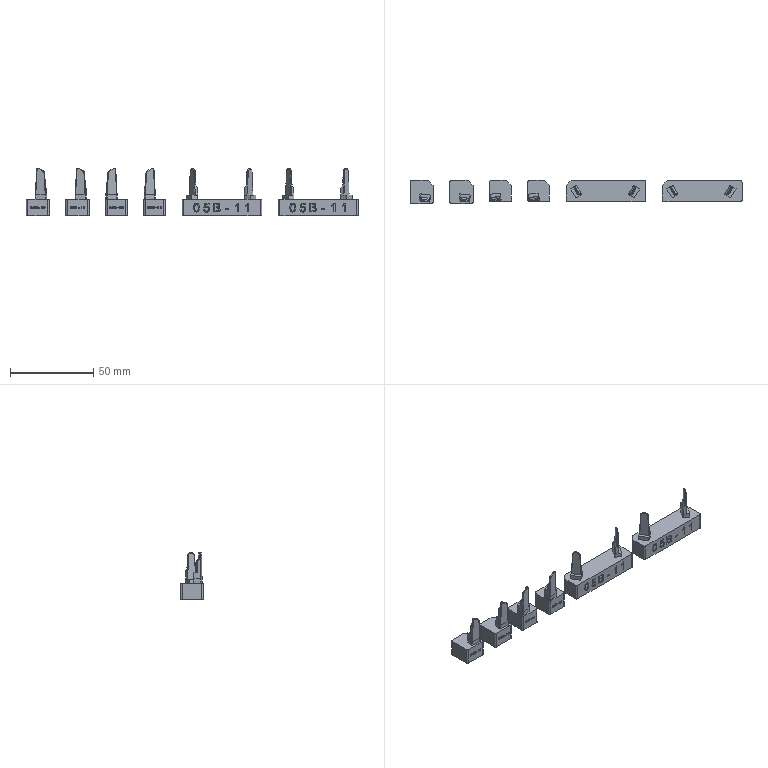NC program | NX | posted with a generic post | part box 200 x 14 x 28.763 mm
Lines 21030 to 21844 of 209396:
(CONTOUR_AREA_0_0 , TOOL : D4R2)
N41980 M6
N41982 G53
N41984 G17 G0 G90 X91.621 Y3.419 S13000 M3
N41986 G43 Z5. H0
N41988 Z2.6
N41990 G94 G1 Z-4.451 F2000.
N41992 X91.634 Y3.432 Z-4.51
N41994 X91.669 Y3.467 Z-4.546
N41996 X91.713 Y3.511 Z-4.547
N41998 X91.748 Y3.546 Z-4.511
N42000 X91.762 Y3.56 Z-4.453
N42002 X91.765 Y3.563 Z-4.28
N42004 X91.773 Y3.571 Z-4.083
N42006 X91.781 Y3.579 Z-3.96
N42008 X91.784 Y3.582 Z-3.927
N42010 X91.805 Y3.603 Z-3.742
N42012 X91.841 Y3.639 Z-3.608
N42014 X91.875 Y3.673 Z-3.541
N42016 X91.909 Y3.707 Z-3.499
N42018 X91.942 Y3.74 Z-3.477
N42020 X91.976 Y3.774 Z-3.468
N42022 X92.043 Y3.841 Z-3.476
N42024 X92.111 Y3.909 Z-3.512
N42026 X92.178 Y3.976 Z-3.582
N42028 X92.246 Y4.044 Z-3.679
N42030 X92.313 Y4.111 Z-3.817
N42032 X92.347 Y4.145 Z-3.917
N42034 X92.38 Y4.178 Z-4.052
N42036 X92.404 Y4.202 Z-4.2
N42038 X92.412 Y4.21 Z-4.274
N42040 X92.422 Y4.22 Z-4.414
N42042 X92.45 Y4.239 Z-4.413
N42044 X92.594 Y4.321 Z-4.406
N42046 X92.579 Y4.307 Z-4.211
N42048 X92.564 Y4.292 Z-4.076
N42050 X92.521 Y4.249 Z-3.857
N42052 X92.478 Y4.206 Z-3.71
N42054 X92.392 Y4.12 Z-3.503
N42056 X92.306 Y4.034 Z-3.355
N42058 X92.22 Y3.948 Z-3.244
N42060 X92.134 Y3.862 Z-3.165
N42062 X92.048 Y3.776 Z-3.112
N42064 X91.962 Y3.69 Z-3.083
N42066 X91.876 Y3.604 Z-3.088
N42068 X91.826 Y3.554 Z-3.107
N42070 X91.776 Y3.504 Z-3.15
N42072 X91.726 Y3.454 Z-3.23
N42074 X91.701 Y3.429 Z-3.298
N42076 X91.676 Y3.404 Z-3.435
N42078 X91.67 Y3.398 Z-3.487
N42080 X91.666 Y3.393 Z-3.539
N42082 X91.664 Y3.391 Z-3.578
N42084 X91.643 Y3.371 Z-4.292
N42086 X91.608 Y3.31 Z-3.934
N42088 X91.572 Y3.25 Z-3.74
N42090 X91.542 Y3.199 Z-3.628
N42092 X91.55 Y3.208 Z-3.334
N42094 X91.554 Y3.212 Z-3.226
N42096 X91.558 Y3.216 Z-3.182
N42098 X91.575 Y3.232 Z-3.081
N42100 X91.596 Y3.253 Z-3.008
N42102 X91.617 Y3.274 Z-2.962
N42104 X91.659 Y3.316 Z-2.898
N42106 X91.701 Y3.359 Z-2.856
N42108 X91.743 Y3.401 Z-2.83
N42110 X91.827 Y3.485 Z-2.805
N42112 X91.911 Y3.569
N42114 X92.011 Y3.668 Z-2.832
N42116 X92.11 Y3.767 Z-2.882
N42118 X92.209 Y3.866 Z-2.959
N42120 X92.308 Y3.965 Z-3.062
N42122 X92.407 Y4.065 Z-3.196
N42124 X92.506 Y4.164 Z-3.373
N42126 X92.605 Y4.263 Z-3.622
N42128 X92.655 Y4.312 Z-3.8
N42130 X92.679 Y4.337 Z-3.915
N42132 X92.704 Y4.362 Z-4.078
N42134 X92.727 Y4.385 Z-4.401
N42136 X92.775 Y4.407 Z-4.398
N42138 X92.847 Y4.435 Z-4.394
N42140 X92.828 Y4.416 Z-4.117
N42142 X92.795 Y4.383 Z-3.873
N42144 X92.742 Y4.33 Z-3.642
N42146 X92.689 Y4.277 Z-3.472
N42148 X92.636 Y4.223 Z-3.338
N42150 X92.583 Y4.17 Z-3.225
N42152 X92.477 Y4.064 Z-3.043
N42154 X92.371 Y3.958 Z-2.9
N42156 X92.265 Y3.852 Z-2.788
N42158 X92.159 Y3.746 Z-2.703
N42160 X92.053 Y3.64 Z-2.64
N42162 X91.947 Y3.534 Z-2.599
N42164 X91.826 Y3.413 Z-2.581
N42166 X91.705 Y3.293 Z-2.597
N42168 X91.645 Y3.232 Z-2.623
N42170 X91.584 Y3.172 Z-2.663
N42172 X91.524 Y3.112 Z-2.734
N42174 X91.494 Y3.081 Z-2.785
N42176 X91.464 Y3.051 Z-2.866
N42178 X91.455 Y3.043 Z-2.904
N42180 X91.447 Y3.034 Z-2.952
N42182 X91.438 Y3.026 Z-3.034
N42184 X91.43 Y3.017 Z-3.328
N42186 X91.315 Y2.833 Z-3.126
N42188 X91.322 Y2.839 Z-2.897
N42190 X91.324 Y2.841 Z-2.857
N42192 X91.332 Y2.85 Z-2.792
N42194 X91.349 Y2.867 Z-2.714
N42196 X91.389 Y2.906 Z-2.62
N42198 X91.428 Y2.946 Z-2.559
N42200 X91.507 Y3.025 Z-2.481
N42202 X91.586 Y3.104 Z-2.435
N42204 X91.665 Y3.183 Z-2.408
N42206 X91.744 Y3.262 Z-2.398
N42208 X91.824 Y3.341 Z-2.399
N42210 X91.982 Y3.499 Z-2.434
N42212 X92.088 Y3.605 Z-2.48
N42214 X92.194 Y3.711 Z-2.545
N42216 X92.3 Y3.817 Z-2.631
N42218 X92.406 Y3.923 Z-2.737
N42220 X92.512 Y4.029 Z-2.87
N42222 X92.618 Y4.135 Z-3.034
N42224 X92.724 Y4.241 Z-3.249
N42226 X92.777 Y4.294 Z-3.381
N42228 X92.83 Y4.347 Z-3.54
N42230 X92.883 Y4.4 Z-3.746
N42232 X92.909 Y4.426 Z-3.885
N42234 X92.935 Y4.453 Z-4.092
N42236 X92.951 Y4.468 Z-4.389
N42238 X93.048 Y4.495 Z-4.386
N42240 X93.032 Y4.479 Z-4.054
N42242 X92.99 Y4.438 Z-3.77
N42244 X92.949 Y4.396 Z-3.582
N42246 X92.865 Y4.312 Z-3.315
N42248 X92.759 Y4.206 Z-3.067
N42250 X92.653 Y4.1 Z-2.875
N42252 X92.547 Y3.994 Z-2.722
N42254 X92.441 Y3.888 Z-2.597
N42256 X92.335 Y3.782 Z-2.494
N42258 X92.229 Y3.676 Z-2.411
N42260 X92.123 Y3.57 Z-2.344
N42262 X92.017 Y3.464 Z-2.294
N42264 X91.919 Y3.366 Z-2.263
N42266 X91.821 Y3.268 Z-2.244
N42268 X91.723 Y3.17 Z-2.239
N42270 X91.625 Y3.072 Z-2.251
N42272 X91.527 Y2.974 Z-2.279
N42274 X91.429 Y2.876 Z-2.333
N42276 X91.331 Y2.778 Z-2.422
N42278 X91.282 Y2.729 Z-2.493
N42280 X91.233 Y2.68 Z-2.603
N42282 X91.214 Y2.661 Z-2.691
N42284 X91.207 Y2.654 Z-2.739
N42286 X91.198 Y2.646 Z-2.999
N42288 X91.126 Y2.531 Z-2.946
N42290 X91.081 Y2.458 Z-2.916
N42292 X91.087 Y2.464 Z-2.689
N42294 X91.089 Y2.466 Z-2.66
N42296 X91.098 Y2.475 Z-2.603
N42298 X91.115 Y2.492 Z-2.527
N42300 X91.159 Y2.536 Z-2.423
N42302 X91.203 Y2.58 Z-2.352
N42304 X91.256 Y2.633 Z-2.289
N42306 X91.309 Y2.686 Z-2.242
N42308 X91.415 Y2.792 Z-2.172
N42310 X91.521 Y2.898 Z-2.13
N42312 X91.628 Y3.005 Z-2.107
N42314 X91.734 Y3.111 Z-2.102
N42316 X91.84 Y3.217 Z-2.111
N42318 X91.946 Y3.323 Z-2.134
N42320 X92.052 Y3.429 Z-2.172
N42322 X92.158 Y3.535 Z-2.224
N42324 X92.264 Y3.641 Z-2.29
N42326 X92.37 Y3.747 Z-2.372
N42328 X92.476 Y3.853 Z-2.473
N42330 X92.582 Y3.959 Z-2.592
N42332 X92.688 Y4.065 Z-2.737
N42334 X92.794 Y4.171 Z-2.914
N42336 X92.9 Y4.277 Z-3.137
N42338 X92.957 Y4.334 Z-3.283
N42340 X93.015 Y4.392 Z-3.461
N42342 X93.072 Y4.449 Z-3.689
N42344 X93.1 Y4.477 Z-3.844
N42346 X93.129 Y4.506 Z-4.08
N42348 X93.144 Y4.521 Z-4.383
N42350 X93.191 Y4.534 Z-4.382
N42352 X93.233 Y4.54 Z-4.381
N42354 X93.22 Y4.527 Z-4.118
N42356 X93.184 Y4.491 Z-3.811
N42358 X93.149 Y4.456 Z-3.624
N42360 X93.078 Y4.385 Z-3.353
N42362 X93.007 Y4.313 Z-3.151
N42364 X92.935 Y4.242 Z-2.985
N42366 X92.829 Y4.136 Z-2.782
N42368 X92.723 Y4.03 Z-2.616
N42370 X92.617 Y3.924 Z-2.477
N42372 X92.511 Y3.818 Z-2.361
N42374 X92.405 Y3.712 Z-2.264
N42376 X92.299 Y3.606 Z-2.182
N42378 X92.193 Y3.5 Z-2.115
N42380 X92.087 Y3.394 Z-2.063
N42382 X91.981 Y3.288 Z-2.023
N42384 X91.875 Y3.182 Z-1.996
N42386 X91.769 Y3.076 Z-1.981
N42388 X91.663 Y2.969
N42390 X91.557 Y2.863 Z-1.992
N42392 X91.45 Y2.757 Z-2.021
N42394 X91.344 Y2.651 Z-2.066
N42396 X91.238 Y2.545 Z-2.134
N42398 X91.118 Y2.424 Z-2.252
N42400 X91.057 Y2.364 Z-2.343
N42402 X91.027 Y2.334 Z-2.4
N42404 X90.997 Y2.304 Z-2.48
N42406 X90.979 Y2.286 Z-2.557
N42408 X90.971 Y2.277 Z-2.614
N42410 X90.968 Y2.275 Z-2.641
N42412 X90.962 Y2.269 Z-2.865
N42414 X90.896 Y2.164 Z-2.844
N42416 X90.873 Y2.128 Z-2.843
N42418 X90.842 Y2.079 Z-2.849
N42420 X90.851 Y2.087 Z-2.597
N42422 X90.857 Y2.094 Z-2.551
N42424 X90.877 Y2.114 Z-2.461
N42426 X90.927 Y2.164 Z-2.337
N42428 X90.976 Y2.213 Z-2.25
N42430 X91.075 Y2.312 Z-2.128
N42432 X91.174 Y2.411 Z-2.04
N42434 X91.273 Y2.51 Z-1.977
N42436 X91.379 Y2.616 Z-1.927
N42438 X91.486 Y2.722 Z-1.894
N42440 X91.592 Y2.828 Z-1.875
N42442 X91.698 Y2.934 Z-1.869
N42444 X91.804 Y3.04 Z-1.876
N42446 X91.91 Y3.146 Z-1.894
N42448 X92.016 Y3.253 Z-1.923
N42450 X92.122 Y3.359 Z-1.965
N42452 X92.228 Y3.465 Z-2.019
N42454 X92.334 Y3.571 Z-2.085
N42456 X92.44 Y3.677 Z-2.165
N42458 X92.546 Y3.783 Z-2.26
N42460 X92.652 Y3.889 Z-2.373
N42462 X92.758 Y3.995 Z-2.506
N42464 X92.864 Y4.101 Z-2.664
N42466 X92.97 Y4.207 Z-2.853
N42468 X93.053 Y4.29 Z-3.032
N42470 X93.136 Y4.372 Z-3.254
N42472 X93.218 Y4.455 Z-3.545
N42474 X93.26 Y4.496 Z-3.749
N42476 X93.301 Y4.538 Z-4.072
N42478 X93.314 Y4.55 Z-4.379
N42480 X93.395 Y4.561 Z-4.377
N42482 X93.382 Y4.548 Z-4.074
N42484 X93.358 Y4.525 Z-3.854
N42486 X93.335 Y4.501 Z-3.707
N42488 X93.288 Y4.454 Z-3.483
N42490 X93.194 Y4.36 Z-3.166
N42492 X93.1 Y4.266 Z-2.93
N42494 X93.006 Y4.172 Z-2.737
N42496 X92.9 Y4.066 Z-2.557
N42498 X92.793 Y3.96 Z-2.407
N42500 X92.687 Y3.854 Z-2.278
N42502 X92.581 Y3.748 Z-2.169
N42504 X92.475 Y3.642 Z-2.074
N42506 X92.369 Y3.536 Z-1.995
N42508 X92.263 Y3.43 Z-1.929
N42510 X92.157 Y3.324 Z-1.876
N42512 X91.945 Y3.111 Z-1.801
N42514 X91.733 Y2.899 Z-1.771
N42516 X91.627 Y2.793 Z-1.772
N42518 X91.521 Y2.687 Z-1.785
N42520 X91.415 Y2.581 Z-1.811
N42522 X91.309 Y2.475 Z-1.848
N42524 X91.171 Y2.337 Z-1.922
N42526 X91.033 Y2.199 Z-2.027
N42528 X90.964 Y2.13 Z-2.099
N42530 X90.895 Y2.061 Z-2.184
N42532 X90.826 Y1.992 Z-2.298
N42534 X90.791 Y1.958 Z-2.371
N42536 X90.757 Y1.923 Z-2.47
N42538 X90.748 Y1.914 Z-2.505
N42540 X90.735 Y1.901 Z-2.577
N42542 X90.73 Y1.897 Z-2.611
N42544 X90.721 Y1.888 Z-2.86
N42546 X90.601 Y1.697 Z-2.877
N42548 X90.61 Y1.706 Z-2.634
N42550 X90.616 Y1.713 Z-2.588
N42552 X90.636 Y1.732 Z-2.494
N42554 X90.68 Y1.777 Z-2.372
N42556 X90.725 Y1.821 Z-2.28
N42558 X90.813 Y1.909 Z-2.14
N42560 X90.901 Y1.998 Z-2.031
N42562 X90.99 Y2.086 Z-1.946
N42564 X91.167 Y2.263 Z-1.82
N42566 X91.344 Y2.44 Z-1.739
N42568 X91.45 Y2.546 Z-1.707
N42570 X91.556 Y2.652 Z-1.688
N42572 X91.768 Y2.864 Z-1.681
N42574 X91.98 Y3.076 Z-1.716
N42576 X92.192 Y3.288 Z-1.792
N42578 X92.298 Y3.395 Z-1.847
N42580 X92.404 Y3.501 Z-1.913
N42582 X92.51 Y3.607 Z-1.991
N42584 X92.616 Y3.713 Z-2.083
N42586 X92.722 Y3.819 Z-2.19
N42588 X92.829 Y3.925 Z-2.315
N42590 X92.935 Y4.031 Z-2.461
N42592 X93.041 Y4.137 Z-2.633
N42594 X93.146 Y4.242 Z-2.837
N42596 X93.252 Y4.348 Z-3.093
N42598 X93.304 Y4.401 Z-3.251
N42600 X93.357 Y4.453 Z-3.44
N42602 X93.41 Y4.506 Z-3.687
N42604 X93.436 Y4.533 Z-3.856
N42606 X93.463 Y4.559 Z-4.126
N42608 X93.475 Y4.572 Z-4.374
N42610 X93.485 Y4.573
N42612 X93.547 Z-4.373
N42614 X93.536 Y4.562 Z-4.105
N42616 X93.507 Y4.533 Z-3.82
N42618 X93.478 Y4.505 Z-3.643
N42620 X93.421 Y4.447 Z-3.386
N42622 X93.363 Y4.39 Z-3.186
N42624 X93.306 Y4.332 Z-3.021
N42626 X93.191 Y4.217 Z-2.752
N42628 X93.076 Y4.102 Z-2.536
N42630 X92.97 Y3.996 Z-2.372
N42632 X92.864 Y3.89 Z-2.232
N42634 X92.758 Y3.784 Z-2.11
N42636 X92.651 Y3.678 Z-2.005
N42638 X92.545 Y3.572 Z-1.914
N42640 X92.439 Y3.466 Z-1.837
N42642 X92.227 Y3.253 Z-1.717
N42644 X92.015 Y3.041 Z-1.639
N42646 X91.803 Y2.829 Z-1.6
N42648 X91.591 Y2.617
N42650 X91.379 Y2.405 Z-1.641
N42652 X91.273 Y2.299 Z-1.679
N42654 X91.167 Y2.193 Z-1.729
N42656 X91.06 Y2.087 Z-1.792
N42658 X90.954 Y1.981 Z-1.872
N42660 X90.848 Y1.875 Z-1.971
N42662 X90.742 Y1.768 Z-2.095
N42664 X90.636 Y1.662 Z-2.248
N42666 X90.583 Y1.609 Z-2.346
N42668 X90.53 Y1.556 Z-2.472
N42670 X90.515 Y1.541 Z-2.521
N42672 X90.495 Y1.521 Z-2.615
N42674 X90.488 Y1.514 Z-2.663
N42676 X90.479 Y1.506 Z-2.916
N42678 X90.393 Y1.369 Z-2.931
N42680 X90.359 Y1.315 Z-2.939
N42682 X90.367 Y1.323 Z-2.689
N42684 X90.374 Y1.33 Z-2.642
N42686 X90.394 Y1.35 Z-2.547
N42688 X90.437 Y1.393 Z-2.428
N42690 X90.48 Y1.436 Z-2.338
N42692 X90.565 Y1.521 Z-2.198
N42694 X90.671 Y1.627 Z-2.058
N42696 X90.777 Y1.733 Z-1.941
N42698 X90.883 Y1.839 Z-1.839
N42700 X90.99 Y1.945 Z-1.754
N42702 X91.096 Y2.052 Z-1.686
N42704 X91.202 Y2.158 Z-1.63
N42706 X91.308 Y2.264 Z-1.587
N42708 X91.414 Y2.37 Z-1.555
N42710 X91.626 Y2.582 Z-1.521
N42712 X91.838 Y2.794 Z-1.525
N42714 X92.05 Y3.006 Z-1.566
N42716 X92.262 Y3.218 Z-1.646
N42718 X92.474 Y3.43 Z-1.765
N42720 X92.58 Y3.536 Z-1.842
N42722 X92.687 Y3.643 Z-1.931
N42724 X92.793 Y3.749 Z-2.034
N42726 X92.899 Y3.855 Z-2.153
N42728 X93.005 Y3.961 Z-2.29
N42730 X93.111 Y4.067 Z-2.45
N42732 X93.235 Y4.191 Z-2.673
N42734 X93.358 Y4.314 Z-2.951
N42736 X93.42 Y4.376 Z-3.123
N42738 X93.482 Y4.438 Z-3.331
N42740 X93.544 Y4.5 Z-3.602
N42742 X93.575 Y4.531 Z-3.787
N42744 X93.606 Y4.562 Z-4.079
N42746 X93.617 Y4.573 Z-4.372
N42748 X93.687 Z-4.37
N42750 X93.676 Y4.562 Z-4.09
N42752 X93.643 Y4.529 Z-3.772
N42754 X93.61 Y4.496 Z-3.576
N42756 X93.544 Y4.429 Z-3.288
N42758 X93.477 Y4.363 Z-3.071
N42760 X93.411 Y4.297 Z-2.891
N42762 X93.278 Y4.164 Z-2.6
N42764 X93.146 Y4.032 Z-2.369
N42766 X93.04 Y3.926 Z-2.214
N42768 X92.934 Y3.82 Z-2.08
N42770 X92.828 Y3.714 Z-1.964
N42772 X92.722 Y3.607 Z-1.863
N42774 X92.51 Y3.395 Z-1.699
N42776 X92.297 Y3.183 Z-1.579
N42778 X92.085 Y2.971 Z-1.499
N42780 X91.873 Y2.759 Z-1.455
N42782 X91.661 Y2.547 Z-1.448
N42784 X91.449 Y2.335 Z-1.476
N42786 X91.237 Y2.123 Z-1.543
N42788 X91.131 Y2.016 Z-1.592
N42790 X91.025 Y1.91 Z-1.653
N42792 X90.919 Y1.804 Z-1.728
N42794 X90.812 Y1.698 Z-1.817
N42796 X90.6 Y1.486 Z-2.027
N42798 X90.437 Y1.322 Z-2.235
N42800 X90.355 Y1.241 Z-2.371
N42802 X90.314 Y1.2 Z-2.458
N42804 X90.273 Y1.159 Z-2.575
N42806 X90.253 Y1.139 Z-2.672
N42808 X90.246 Y1.132 Z-2.72
N42810 X90.237 Y1.123 Z-2.973
N42812 X90.133 Y0.959 Z-3.021
N42814 X90.13 Y0.953 Z-3.043
N42816 X90.125 Y0.947 Z-3.044
N42818 X90.115 Y0.931 Z-3.039
N42820 X90.124 Y0.94 Z-2.781
N42822 X90.131 Y0.947 Z-2.728
N42824 X90.151 Y0.967 Z-2.625
N42826 X90.212 Y1.027 Z-2.452
N42828 X90.272 Y1.088 Z-2.331
N42830 X90.393 Y1.209 Z-2.155
N42832 X90.514 Y1.33 Z-2.016
N42834 X90.635 Y1.451 Z-1.894
N42836 X90.848 Y1.663 Z-1.712
N42838 X90.954 Y1.769 Z-1.631
N42840 X91.06 Y1.875 Z-1.564
N42842 X91.272 Y2.087 Z-1.463
N42844 X91.484 Y2.3 Z-1.403
N42846 X91.696 Y2.512 Z-1.38
N42848 X91.908 Y2.724 Z-1.391
N42850 X92.12 Y2.936 Z-1.436
N42852 X92.332 Y3.148 Z-1.517
N42854 X92.545 Y3.36 Z-1.637
N42856 X92.757 Y3.572 Z-1.799
N42858 X92.863 Y3.678 Z-1.899
N42860 X92.969 Y3.785 Z-2.014
N42862 X93.075 Y3.891 Z-2.145
N42864 X93.181 Y3.997 Z-2.295
N42866 X93.322 Y4.138 Z-2.535
N42868 X93.393 Y4.209 Z-2.677
N42870 X93.464 Y4.279 Z-2.839
N42872 X93.534 Y4.35 Z-3.028
N42874 X93.605 Y4.421 Z-3.255
N42876 X93.676 Y4.491 Z-3.559
N42878 X93.711 Y4.527 Z-3.768
N42880 X93.746 Y4.562 Z-4.122
N42882 X93.757 Y4.573 Z-4.369
N42884 X93.78 Z-4.368
N42886 X93.822 Y4.567
N42888 X93.812 Y4.558 Z-4.122
N42890 X93.794 Y4.539 Z-3.9
N42892 X93.775 Y4.52 Z-3.75
N42894 X93.738 Y4.483 Z-3.531
N42896 X93.663 Y4.409 Z-3.217
N42898 X93.589 Y4.334 Z-2.981
N42900 X93.514 Y4.26 Z-2.785
N42902 X93.44 Y4.185 Z-2.618
N42904 X93.365 Y4.111 Z-2.472
N42906 X93.216 Y3.962 Z-2.225
N42908 X93.11 Y3.855 Z-2.078
N42910 X93.004 Y3.749 Z-1.95
N42912 X92.792 Y3.537 Z-1.739
N42914 X92.58 Y3.325 Z-1.578
N42916 X92.368 Y3.113 Z-1.46
N42918 X92.155 Y2.901 Z-1.377
N42920 X91.943 Y2.689 Z-1.33
N42922 X91.731 Y2.477 Z-1.316
N42924 X91.519 Y2.265 Z-1.336
N42926 X91.307 Y2.052 Z-1.391
N42928 X91.095 Y1.84 Z-1.483
N42930 X90.883 Y1.628 Z-1.618
N42932 X90.67 Y1.416 Z-1.783
N42934 X90.51 Y1.255 Z-1.925
N42936 X90.349 Y1.095 Z-2.09
N42938 X90.269 Y1.014 Z-2.191
N42940 X90.188 Y0.934 Z-2.313
N42942 X90.108 Y0.853 Z-2.471
N42944 X90.068 Y0.813 Z-2.573
N42946 X90.028 Y0.773 Z-2.709
N42948 X90.01 Y0.755 Z-2.809
N42950 X90.001 Y0.746 Z-2.885
N42952 X89.998 Y0.744 Z-2.93
N42954 X89.991 Y0.737 Z-3.166
N42956 X89.947 Y0.667 Z-3.218
N42958 X89.933 Y0.646 Z-3.23
N42960 X89.866 Y0.542 Z-3.339
N42962 X89.876 Y0.551 Z-3.037
N42964 X89.88 Y0.555 Z-2.982
N42966 X89.885 Y0.56 Z-2.946
N42968 X89.903 Y0.578 Z-2.832
N42970 X89.953 Y0.628 Z-2.648
N42972 X90.003 Y0.679 Z-2.514
N42974 X90.104 Y0.779 Z-2.316
N42976 X90.204 Y0.879 Z-2.161
N42978 X90.304 Y0.98 Z-2.039
N42980 X90.405 Y1.08 Z-1.936
N42982 X90.505 Y1.18 Z-1.847
N42984 X90.706 Y1.381 Z-1.686
N42986 X90.918 Y1.593 Z-1.535
N42988 X91.13 Y1.805 Z-1.409
N42990 X91.342 Y2.017 Z-1.324
N42992 X91.554 Y2.229 Z-1.274
N42994 X91.766 Y2.442 Z-1.257
N42996 X91.978 Y2.654 Z-1.273
N42998 X92.19 Y2.866 Z-1.322
N43000 X92.403 Y3.078 Z-1.404
N43002 X92.615 Y3.29 Z-1.522
N43004 X92.827 Y3.502 Z-1.682
N43006 X92.933 Y3.608 Z-1.779
N43008 X93.039 Y3.714 Z-1.89
N43010 X93.145 Y3.82 Z-2.016
N43012 X93.251 Y3.926 Z-2.16
N43014 X93.407 Y4.082 Z-2.412
N43016 X93.485 Y4.16 Z-2.562
N43018 X93.563 Y4.238 Z-2.732
N43020 X93.64 Y4.316 Z-2.932
N43022 X93.718 Y4.394 Z-3.176
N43024 X93.796 Y4.471 Z-3.497
N43026 X93.835 Y4.51 Z-3.721
N43028 X93.855 Y4.53 Z-3.871
N43030 X93.874 Y4.549 Z-4.094
N43032 X93.884 Y4.559 Z-4.367
N43034 X93.946 Y4.551 Z-4.366
N43036 X93.936 Y4.541 Z-4.085
N43038 X93.915 Y4.521 Z-3.856
N43040 X93.895 Y4.5 Z-3.703
N43042 X93.855 Y4.46 Z-3.472
N43044 X93.773 Y4.379 Z-3.142
N43046 X93.692 Y4.297 Z-2.89
N43048 X93.611 Y4.216 Z-2.686
N43050 X93.53 Y4.135 Z-2.511
N43052 X93.449 Y4.054 Z-2.358
N43054 X93.286 Y3.891 Z-2.1
N43056 X93.18 Y3.785 Z-1.959
N43058 X93.074 Y3.679 Z-1.835
N43060 X92.862 Y3.467 Z-1.629
N43062 X92.65 Y3.255 Z-1.471
N43064 X92.438 Y3.043 Z-1.352
N43066 X92.226 Y2.831 Z-1.27
N43068 X92.013 Y2.619 Z-1.22
N43070 X91.801 Y2.406 Z-1.201
N43072 X91.589 Y2.194 Z-1.215
N43074 X91.377 Y1.982 Z-1.261
N43076 X91.165 Y1.77 Z-1.342
N43078 X90.953 Y1.558 Z-1.459
N43080 X90.741 Y1.346 Z-1.599
N43082 X90.529 Y1.134 Z-1.755
N43084 X90.316 Y0.922 Z-1.938
N43086 X90.21 Y0.815 Z-2.055
N43088 X90.104 Y0.709 Z-2.196
N43090 X89.998 Y0.603 Z-2.371
N43092 X89.892 Y0.497 Z-2.598
N43094 X89.834 Y0.439 Z-2.768
N43096 X89.805 Y0.41 Z-2.872
N43098 X89.776 Y0.381 Z-3.011
N43100 X89.757 Y0.362 Z-3.149
N43102 X89.752 Y0.358 Z-3.199
N43104 X89.748 Y0.353 Z-3.295
N43106 X89.738 Y0.343 Z-3.62
N43108 X89.7 Y0.284 Z-3.746
N43110 X89.652 Y0.212 Z-3.938
N43112 X89.628 Y0.176 Z-4.09
N43114 X89.603 Y0.14 Z-4.313
N43116 X89.598 Y0.133 Z-4.334
N43118 X89.62 Y0.155 Z-3.581
N43120 X89.625 Y0.16 Z-3.477
N43122 X89.633 Y0.168 Z-3.385
N43124 X89.641 Y0.176 Z-3.309
N43126 X89.677 Y0.212 Z-3.085
N43128 X89.713 Y0.248 Z-2.934
N43130 X89.784 Y0.319 Z-2.703
N43132 X89.856 Y0.391 Z-2.528
N43134 X89.927 Y0.462 Z-2.381
N43136 X90.033 Y0.568 Z-2.204
N43138 X90.139 Y0.674 Z-2.057
N43140 X90.245 Y0.78 Z-1.935
N43142 X90.351 Y0.886 Z-1.832
N43144 X90.564 Y1.099 Z-1.665
N43146 X90.776 Y1.311 Z-1.521
N43148 X90.988 Y1.523 Z-1.39
N43150 X91.2 Y1.735 Z-1.279
N43152 X91.412 Y1.947 Z-1.203
N43154 X91.624 Y2.159 Z-1.16
N43156 X91.836 Y2.371 Z-1.15
N43158 X92.049 Y2.584 Z-1.17
N43160 X92.261 Y2.796 Z-1.22
N43162 X92.473 Y3.008 Z-1.303
N43164 X92.685 Y3.22 Z-1.422
N43166 X92.897 Y3.432 Z-1.579
N43168 X93.109 Y3.644 Z-1.783
N43170 X93.215 Y3.75 Z-1.905
N43172 X93.321 Y3.856 Z-2.043
N43174 X93.49 Y4.025 Z-2.307
N43176 X93.575 Y4.11 Z-2.464
N43178 X93.659 Y4.194 Z-2.645
N43180 X93.744 Y4.279 Z-2.855
N43182 X93.829 Y4.364 Z-3.112
N43184 X93.913 Y4.448 Z-3.452
N43186 X93.955 Y4.49 Z-3.692
N43188 X93.976 Y4.511 Z-3.853
N43190 X93.998 Y4.533 Z-4.098
N43192 X94.007 Y4.542 Z-4.366
N43194 X94.069 Y4.534 Z-4.357
N43196 X94.059 Y4.524 Z-4.139
N43198 X94.037 Y4.502 Z-3.866
N43200 X94.015 Y4.48 Z-3.694
N43202 X93.972 Y4.436 Z-3.441
N43204 X93.884 Y4.348 Z-3.088
N43206 X93.796 Y4.261 Z-2.823
N43208 X93.708 Y4.173 Z-2.606
N43210 X93.62 Y4.085 Z-2.421
N43212 X93.532 Y3.997 Z-2.259
N43214 X93.356 Y3.821 Z-1.989
N43216 X93.25 Y3.715 Z-1.852
N43218 X93.144 Y3.609 Z-1.732
N43220 X92.932 Y3.397 Z-1.531
N43222 X92.72 Y3.185 Z-1.375
N43224 X92.508 Y2.973 Z-1.258
N43226 X92.296 Y2.761 Z-1.174
N43228 X92.084 Y2.548 Z-1.122
N43230 X91.871 Y2.336 Z-1.101
N43232 X91.659 Y2.124 Z-1.109
N43234 X91.447 Y1.912 Z-1.149
N43236 X91.235 Y1.7 Z-1.22
N43238 X91.023 Y1.488 Z-1.326
N43240 X90.811 Y1.276 Z-1.449
N43242 X90.599 Y1.064 Z-1.584
N43244 X90.387 Y0.851 Z-1.737
N43246 X90.28 Y0.745 Z-1.832
N43248 X90.174 Y0.639 Z-1.942
N43250 X90.068 Y0.533 Z-2.071
N43252 X89.962 Y0.427 Z-2.226
N43254 X89.851 Y0.316 Z-2.419
N43256 X89.74 Y0.205 Z-2.665
N43258 X89.685 Y0.149 Z-2.815
N43260 X89.629 Y0.094 Z-2.999
N43262 X89.573 Y0.038 Z-3.241
N43264 X89.546 Y0.01 Z-3.399
N43266 X89.518 Y-0.017 Z-3.62
N43268 X89.5 Y-0.035 Z-3.844
N43270 X89.494 Y-0.041 Z-3.94
N43272 X89.486 Y-0.049 Z-4.111
N43274 Z-4.546
N43276 X89.384 Y-0.222 Z-4.536
N43278 X89.392 Y-0.214 Z-4.29
N43280 X89.4 Y-0.206 Z-4.122
N43282 X89.415 Y-0.19 Z-3.902
N43284 X89.452 Y-0.154 Z-3.585
N43286 X89.488 Y-0.117 Z-3.363
N43288 X89.561 Y-0.045 Z-3.047
N43290 X89.634 Y0.028 Z-2.814
N43292 X89.706 Y0.101 Z-2.624
N43294 X89.779 Y0.174 Z-2.465
N43296 X89.852 Y0.247 Z-2.328
N43298 X89.997 Y0.392 Z-2.097
N43300 X90.103 Y0.498 Z-1.961
N43302 X90.21 Y0.604 Z-1.842
N43304 X90.316 Y0.71 Z-1.741
N43306 X90.422 Y0.816 Z-1.653
N43308 X90.634 Y1.028 Z-1.51
N43310 X90.846 Y1.241 Z-1.384
N43312 X91.058 Y1.453 Z-1.266
N43314 X91.27 Y1.665 Z-1.166
N43316 X91.482 Y1.877 Z-1.098
N43318 X91.694 Y2.089 Z-1.061
N43320 X91.907 Y2.301 Z-1.055
N43322 X92.119 Y2.513 Z-1.077
N43324 X92.331 Y2.725 Z-1.13
N43326 X92.543 Y2.938 Z-1.214
N43328 X92.755 Y3.15 Z-1.331
N43330 X92.967 Y3.362 Z-1.486
N43332 X93.179 Y3.574 Z-1.685
N43334 X93.285 Y3.68 Z-1.804
N43336 X93.391 Y3.786 Z-1.939
N43338 X93.573 Y3.967 Z-2.213
N43340 X93.663 Y4.058 Z-2.377
N43342 X93.754 Y4.148 Z-2.565
N43344 X93.844 Y4.239 Z-2.787
N43346 X93.935 Y4.329 Z-3.055
N43348 X93.98 Y4.375 Z-3.219
N43350 X94.025 Y4.42 Z-3.415
N43352 X94.071 Y4.465 Z-3.672
N43354 X94.093 Y4.488 Z-3.846
N43356 X94.116 Y4.511 Z-4.119
N43358 X94.125 Y4.519 Z-4.365
N43360 X94.18 Y4.504 Z-4.364
N43362 X94.171 Y4.495 Z-4.089
N43364 X94.148 Y4.472 Z-3.819
N43366 X94.124 Y4.449 Z-3.647
N43368 X94.078 Y4.402 Z-3.389
N43370 X94.031 Y4.356 Z-3.192
N43372 X93.985 Y4.309 Z-3.025
N43374 X93.892 Y4.216 Z-2.752
N43376 X93.799 Y4.123 Z-2.527
N43378 X93.706 Y4.03 Z-2.336
N43380 X93.613 Y3.937 Z-2.17
N43382 X93.427 Y3.751 Z-1.892
N43384 X93.321 Y3.645 Z-1.759
N43386 X93.214 Y3.539 Z-1.641
N43388 X93.002 Y3.327 Z-1.444
N43390 X92.79 Y3.115 Z-1.29
N43392 X92.578 Y2.903 Z-1.173
N43394 X92.366 Y2.69 Z-1.088
N43396 X92.154 Y2.478 Z-1.035
N43398 X91.942 Y2.266 Z-1.011
N43400 X91.73 Y2.054 Z-1.016
N43402 X91.517 Y1.842 Z-1.05
N43404 X91.305 Y1.63 Z-1.115
N43406 X91.093 Y1.418 Z-1.211
N43408 X90.881 Y1.205 Z-1.322
N43410 X90.669 Y0.993 Z-1.442
N43412 X90.457 Y0.781 Z-1.576
N43414 X90.245 Y0.569 Z-1.754
N43416 X90.139 Y0.463 Z-1.863
N43418 X90.032 Y0.357 Z-1.99
N43420 X89.861 Y0.186 Z-2.238
N43422 X89.776 Y0.1 Z-2.389
N43424 X89.69 Y0.015 Z-2.565
N43426 X89.605 Y-0.071 Z-2.772
N43428 X89.519 Y-0.156 Z-3.032
N43430 X89.434 Y-0.242 Z-3.383
N43432 X89.391 Y-0.284 Z-3.627
N43434 X89.348 Y-0.327 Z-4.
N43436 X89.338 Y-0.337 Z-4.139
N43438 X89.331 Y-0.345 Z-4.289
N43440 X89.329 Y-0.347 Z-4.534
N43442 X89.281 Y-0.465 Z-4.526
N43444 X89.284 Y-0.462 Z-4.324
N43446 X89.291 Y-0.455 Z-4.168
N43448 X89.301 Y-0.445 Z-4.029
N43450 X89.349 Y-0.397 Z-3.631
N43452 X89.397 Y-0.349 Z-3.368
N43454 X89.445 Y-0.301 Z-3.165
N43456 X89.493 Y-0.253 Z-2.996
N43458 X89.588 Y-0.157 Z-2.722
N43460 X89.684 Y-0.061 Z-2.499
N43462 X89.78 Y0.034 Z-2.314
N43464 X89.876 Y0.13 Z-2.156
N43466 X89.972 Y0.226 Z-2.016
N43468 X90.068 Y0.322 Z-1.895
N43470 X90.174 Y0.428 Z-1.777
N43472 X90.28 Y0.534 Z-1.674
N43474 X90.492 Y0.746 Z-1.507
N43476 X90.704 Y0.958 Z-1.38
N43478 X90.916 Y1.17 Z-1.266
N43480 X91.128 Y1.383 Z-1.159
N43482 X91.34 Y1.595 Z-1.067
N43484 X91.552 Y1.807 Z-1.005
N43486 X91.765 Y2.019 Z-0.973
N43488 X91.977 Y2.231 Z-0.97
N43490 X92.189 Y2.443 Z-0.995
N43492 X92.401 Y2.655 Z-1.049
N43494 X92.613 Y2.867 Z-1.134
N43496 X92.825 Y3.08 Z-1.25
N43498 X93.037 Y3.292 Z-1.404
N43500 X93.25 Y3.504 Z-1.601
N43502 X93.356 Y3.61 Z-1.717
N43504 X93.462 Y3.716 Z-1.848
N43506 X93.557 Y3.812 Z-1.981
N43508 X93.653 Y3.907 Z-2.13
N43510 X93.748 Y4.003 Z-2.299
N43512 X93.844 Y4.098 Z-2.493
N43514 X93.939 Y4.194 Z-2.721
N43516 X94.035 Y4.289 Z-2.999
N43518 X94.083 Y4.337 Z-3.169
N43520 X94.13 Y4.385 Z-3.37
N43522 X94.178 Y4.432 Z-3.631
N43524 X94.202 Y4.456 Z-3.806
N43526 X94.226 Y4.48 Z-4.081
N43528 X94.235 Y4.489 Z-4.364
N43530 X94.29 Y4.474
N43532 X94.281 Y4.465 Z-4.095
N43534 X94.256 Y4.441 Z-3.806
N43536 X94.232 Y4.416 Z-3.624
N43538 X94.183 Y4.367 Z-3.356
N43540 X94.134 Y4.318 Z-3.151
N43542 X94.085 Y4.269 Z-2.978
N43544 X93.987 Y4.171 Z-2.693
N43546 X93.889 Y4.073 Z-2.461
N43548 X93.791 Y3.975 Z-2.265
N43550 X93.693 Y3.877 Z-2.093
N43552 X93.595 Y3.779 Z-1.941
N43554 X93.497 Y3.681 Z-1.806
N43556 X93.391 Y3.575 Z-1.676
N43558 X93.285 Y3.469 Z-1.561
N43560 X93.072 Y3.257 Z-1.367
N43562 X92.86 Y3.044 Z-1.213
N43564 X92.648 Y2.832 Z-1.096
N43566 X92.436 Y2.62 Z-1.012
N43568 X92.224 Y2.408 Z-0.957
N43570 X92.012 Y2.196 Z-0.931
N43572 X91.8 Y1.984 Z-0.933
N43574 X91.588 Y1.772 Z-0.962
N43576 X91.375 Y1.56 Z-1.022
N43578 X91.163 Y1.347 Z-1.111
N43580 X90.951 Y1.135 Z-1.213
N43582 X90.739 Y0.923 Z-1.321
N43584 X90.527 Y0.711 Z-1.443
N43586 X90.315 Y0.499 Z-1.602
N43588 X90.209 Y0.393 Z-1.699
N43590 X90.103 Y0.287 Z-1.811
N43592 X89.998 Y0.182 Z-1.936
N43594 X89.893 Y0.077 Z-2.08
N43596 X89.788 Y-0.028 Z-2.246
N43598 X89.682 Y-0.133 Z-2.441
N43600 X89.577 Y-0.238 Z-2.673
N43602 X89.472 Y-0.343 Z-2.964